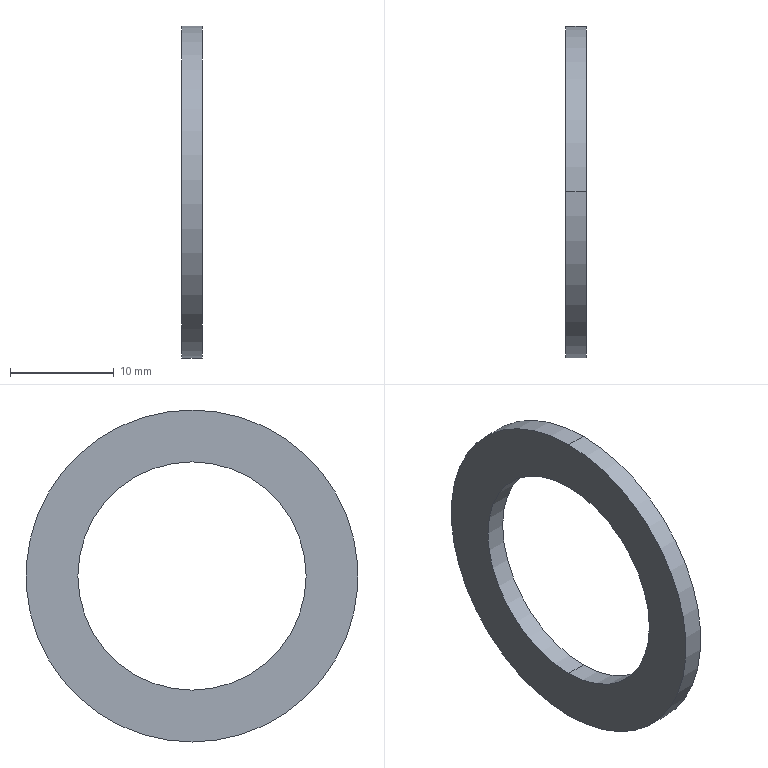Part | SolidWorks | features Revolution 1 | 1 solid | 6 faces | box 2 x 32 x 32 mm | volume 848.23 mm3 | cylinder 4 | plane 2 | commonest cylinder face diameters 22 x2 32 x2
STEP:
#1=CARTESIAN_POINT('',(0.,0.,11.));
#2=VERTEX_POINT('',#1);
#3=CARTESIAN_POINT('',(0.,0.,-11.));
#4=VERTEX_POINT('',#3);
#5=CARTESIAN_POINT('',(0.,0.,0.));
#6=DIRECTION('',(1.,0.,0.));
#7=DIRECTION('',(0.,0.,-1.));
#8=AXIS2_PLACEMENT_3D('',#5,#6,#7);
#9=CIRCLE('',#8,11.);
#10=EDGE_CURVE('',#2,#4,#9,.T.);
#11=ORIENTED_EDGE('',*,*,#10,.F.);
#12=CARTESIAN_POINT('',(2.,0.,11.));
#13=VERTEX_POINT('',#12);
#14=CARTESIAN_POINT('',(0.,0.,11.));
#15=DIRECTION('',(1.,0.,0.));
#16=VECTOR('',#15,1000.);
#17=LINE('',#14,#16);
#18=EDGE_CURVE('',#2,#13,#17,.T.);
#19=ORIENTED_EDGE('',*,*,#18,.T.);
#20=CARTESIAN_POINT('',(2.,0.,-11.));
#21=VERTEX_POINT('',#20);
#22=CARTESIAN_POINT('',(2.,0.,0.));
#23=DIRECTION('',(1.,0.,0.));
#24=DIRECTION('',(0.,0.,-1.));
#25=AXIS2_PLACEMENT_3D('',#22,#23,#24);
#26=CIRCLE('',#25,11.);
#27=EDGE_CURVE('',#13,#21,#26,.T.);
#28=ORIENTED_EDGE('',*,*,#27,.T.);
#29=CARTESIAN_POINT('',(0.,0.,-11.));
#30=DIRECTION('',(1.,0.,0.));
#31=VECTOR('',#30,1000.);
#32=LINE('',#29,#31);
#33=EDGE_CURVE('',#4,#21,#32,.T.);
#34=ORIENTED_EDGE('',*,*,#33,.F.);
#35=EDGE_LOOP('',(#11,#19,#28,#34));
#36=FACE_OUTER_BOUND('',#35,.T.);
#37=CARTESIAN_POINT('',(0.,0.,0.));
#38=DIRECTION('',(1.,0.,0.));
#39=DIRECTION('',(0.,0.,-1.));
#40=AXIS2_PLACEMENT_3D('',#37,#38,#39);
#41=CYLINDRICAL_SURFACE('',#40,11.);
#42=ADVANCED_FACE('',(#36),#41,.F.);
#43=CARTESIAN_POINT('',(0.,0.,-16.));
#44=VERTEX_POINT('',#43);
#45=CARTESIAN_POINT('',(0.,0.,16.));
#46=VERTEX_POINT('',#45);
#47=CARTESIAN_POINT('',(0.,0.,0.));
#48=DIRECTION('',(1.,0.,0.));
#49=DIRECTION('',(0.,0.,-1.));
#50=AXIS2_PLACEMENT_3D('',#47,#48,#49);
#51=CIRCLE('',#50,16.);
#52=EDGE_CURVE('',#44,#46,#51,.T.);
#53=ORIENTED_EDGE('',*,*,#52,.T.);
#54=CARTESIAN_POINT('',(2.,0.,16.));
#55=VERTEX_POINT('',#54);
#56=CARTESIAN_POINT('',(0.,0.,16.));
#57=DIRECTION('',(1.,0.,0.));
#58=VECTOR('',#57,1000.);
#59=LINE('',#56,#58);
#60=EDGE_CURVE('',#46,#55,#59,.T.);
#61=ORIENTED_EDGE('',*,*,#60,.T.);
#62=CARTESIAN_POINT('',(2.,0.,-16.));
#63=VERTEX_POINT('',#62);
#64=CARTESIAN_POINT('',(2.,0.,0.));
#65=DIRECTION('',(1.,0.,0.));
#66=DIRECTION('',(0.,0.,-1.));
#67=AXIS2_PLACEMENT_3D('',#64,#65,#66);
#68=CIRCLE('',#67,16.);
#69=EDGE_CURVE('',#63,#55,#68,.T.);
#70=ORIENTED_EDGE('',*,*,#69,.F.);
#71=CARTESIAN_POINT('',(0.,0.,-16.));
#72=DIRECTION('',(1.,0.,0.));
#73=VECTOR('',#72,1000.);
#74=LINE('',#71,#73);
#75=EDGE_CURVE('',#44,#63,#74,.T.);
#76=ORIENTED_EDGE('',*,*,#75,.F.);
#77=EDGE_LOOP('',(#53,#61,#70,#76));
#78=FACE_OUTER_BOUND('',#77,.T.);
#79=CARTESIAN_POINT('',(0.,0.,0.));
#80=DIRECTION('',(1.,0.,0.));
#81=DIRECTION('',(0.,0.,-1.));
#82=AXIS2_PLACEMENT_3D('',#79,#80,#81);
#83=CYLINDRICAL_SURFACE('',#82,16.);
#84=ADVANCED_FACE('',(#78),#83,.T.);
#85=CARTESIAN_POINT('',(0.,0.,0.));
#86=DIRECTION('',(1.,0.,0.));
#87=DIRECTION('',(0.,0.,-1.));
#88=AXIS2_PLACEMENT_3D('',#85,#86,#87);
#89=CIRCLE('',#88,11.);
#90=EDGE_CURVE('',#4,#2,#89,.T.);
#91=ORIENTED_EDGE('',*,*,#90,.T.);
#92=ORIENTED_EDGE('',*,*,#10,.T.);
#93=EDGE_LOOP('',(#91,#92));
#94=FACE_BOUND('',#93,.T.);
#95=ORIENTED_EDGE('',*,*,#52,.F.);
#96=CARTESIAN_POINT('',(0.,0.,0.));
#97=DIRECTION('',(1.,0.,0.));
#98=DIRECTION('',(0.,0.,-1.));
#99=AXIS2_PLACEMENT_3D('',#96,#97,#98);
#100=CIRCLE('',#99,16.);
#101=EDGE_CURVE('',#46,#44,#100,.T.);
#102=ORIENTED_EDGE('',*,*,#101,.F.);
#103=EDGE_LOOP('',(#95,#102));
#104=FACE_OUTER_BOUND('',#103,.T.);
#105=CARTESIAN_POINT('',(0.,11.,0.));
#106=DIRECTION('',(-1.,0.,0.));
#107=DIRECTION('',(0.,0.,1.));
#108=AXIS2_PLACEMENT_3D('',#105,#106,#107);
#109=PLANE('',#108);
#110=ADVANCED_FACE('',(#94,#104),#109,.T.);
#111=ORIENTED_EDGE('',*,*,#60,.F.);
#112=ORIENTED_EDGE('',*,*,#101,.T.);
#113=ORIENTED_EDGE('',*,*,#75,.T.);
#114=CARTESIAN_POINT('',(2.,0.,0.));
#115=DIRECTION('',(1.,0.,0.));
#116=DIRECTION('',(0.,0.,-1.));
#117=AXIS2_PLACEMENT_3D('',#114,#115,#116);
#118=CIRCLE('',#117,16.);
#119=EDGE_CURVE('',#55,#63,#118,.T.);
#120=ORIENTED_EDGE('',*,*,#119,.F.);
#121=EDGE_LOOP('',(#111,#112,#113,#120));
#122=FACE_OUTER_BOUND('',#121,.T.);
#123=CARTESIAN_POINT('',(0.,0.,0.));
#124=DIRECTION('',(1.,0.,0.));
#125=DIRECTION('',(0.,0.,-1.));
#126=AXIS2_PLACEMENT_3D('',#123,#124,#125);
#127=CYLINDRICAL_SURFACE('',#126,16.);
#128=ADVANCED_FACE('',(#122),#127,.T.);
#129=ORIENTED_EDGE('',*,*,#69,.T.);
#130=ORIENTED_EDGE('',*,*,#119,.T.);
#131=EDGE_LOOP('',(#129,#130));
#132=FACE_OUTER_BOUND('',#131,.T.);
#133=CARTESIAN_POINT('',(2.,0.,0.));
#134=DIRECTION('',(1.,0.,0.));
#135=DIRECTION('',(0.,0.,-1.));
#136=AXIS2_PLACEMENT_3D('',#133,#134,#135);
#137=CIRCLE('',#136,11.);
#138=EDGE_CURVE('',#21,#13,#137,.T.);
#139=ORIENTED_EDGE('',*,*,#138,.F.);
#140=ORIENTED_EDGE('',*,*,#27,.F.);
#141=EDGE_LOOP('',(#139,#140));
#142=FACE_BOUND('',#141,.T.);
#143=CARTESIAN_POINT('',(2.,11.,0.));
#144=DIRECTION('',(1.,0.,0.));
#145=DIRECTION('',(0.,0.,-1.));
#146=AXIS2_PLACEMENT_3D('',#143,#144,#145);
#147=PLANE('',#146);
#148=ADVANCED_FACE('',(#132,#142),#147,.T.);
#149=ORIENTED_EDGE('',*,*,#18,.F.);
#150=ORIENTED_EDGE('',*,*,#90,.F.);
#151=ORIENTED_EDGE('',*,*,#33,.T.);
#152=ORIENTED_EDGE('',*,*,#138,.T.);
#153=EDGE_LOOP('',(#149,#150,#151,#152));
#154=FACE_OUTER_BOUND('',#153,.T.);
#155=CARTESIAN_POINT('',(0.,0.,0.));
#156=DIRECTION('',(1.,0.,0.));
#157=DIRECTION('',(0.,0.,-1.));
#158=AXIS2_PLACEMENT_3D('',#155,#156,#157);
#159=CYLINDRICAL_SURFACE('',#158,11.);
#160=ADVANCED_FACE('',(#154),#159,.F.);
#161=CLOSED_SHELL('',(#42,#84,#110,#128,#148,#160));
#162=MANIFOLD_SOLID_BREP('',#161);
#163=CARTESIAN_POINT('',(0.,0.,0.));
#164=DIRECTION('',(0.,0.,1.));
#165=DIRECTION('',(1.,0.,0.));
#166=AXIS2_PLACEMENT_3D('',#163,#164,#165);
#167=(LENGTH_UNIT()NAMED_UNIT(*)SI_UNIT(.MILLI.,.METRE.));
#168=UNCERTAINTY_MEASURE_WITH_UNIT(LENGTH_MEASURE(0.00001),#167,'','');
#169=(NAMED_UNIT(*)PLANE_ANGLE_UNIT()SI_UNIT($,.RADIAN.));
#170=(NAMED_UNIT(*)SI_UNIT($,.STERADIAN.)SOLID_ANGLE_UNIT());
#171=(GEOMETRIC_REPRESENTATION_CONTEXT(3)GLOBAL_UNCERTAINTY_ASSIGNED_CONTEXT((#168))GLOBAL_UNIT_ASSIGNED_CONTEXT((#167,#169,#170))REPRESENTATION_CONTEXT('',''));
#172=ADVANCED_BREP_SHAPE_REPRESENTATION('',(#162,#166),#171);